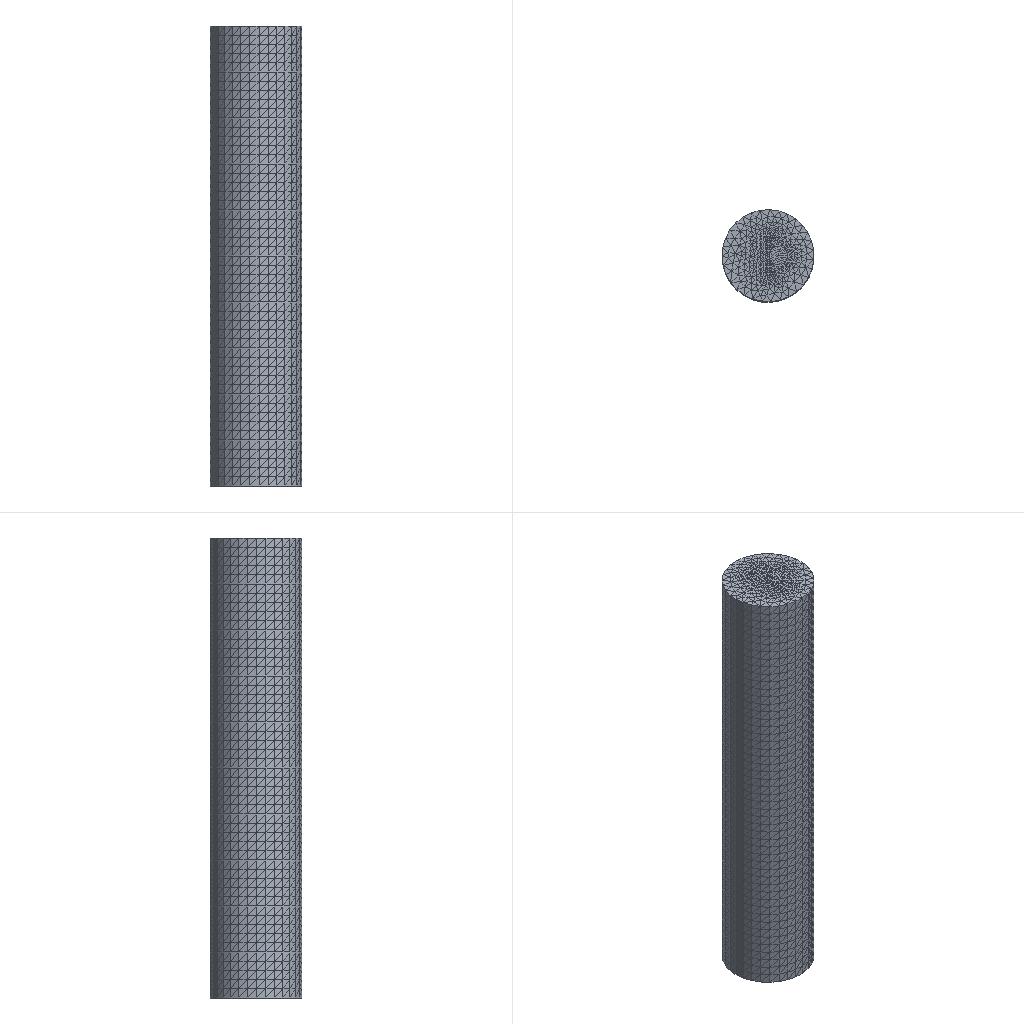Simulation study | abaqus
Set-up summary:
category,name,step,type,value,unit,region
solver,abaqus
solver,version,,,Abaqus/Explicit 2020
units,not stated in the deck,,not stated
analysis,deck,,transient,transient
load_step,Step-1,Step-1,transient,nlgeom=True
contact,interactions,,,general=0 pairs=0 ties=1
load_step,requested,,,1
mesh,nodes,,,13937
mesh,elements,,,62317
element_type,S3,,shell,32
element_type,S4R,,shell,2492
element_type,C3D4,,solid,59793
load,load commands in deck,,count,1
bc,support commands in deck,,count,4
material,BAN,,in results
material,MATERIAL-1,,in results
material,NANG,,in results
check,setup vs results,,match,"per instance, exact: element labels, types and connectivity; labels of the nodes the elements use; coordinates of those nodes at SINGLE_PRECISION in 1 of 5 instance(s)"
Abaqus input file, long lists of numbers shortened:
*Heading
** Job name: Job-2 Model name: Model-1-Copy
** Generated by: Abaqus/CAE 2020
*Preprint, echo=NO, model=NO, history=NO, contact=NO
**
** PARTS
**
*Part, name=qiao
*Node
      1, 0.02, -0.1,           0.
      2, 0.02,           0.,           0.
** (627 more lines like these left out)
*Element, type=S4R
  1,   1,  28,  78,  29
  2,  28,  27,  79,  78
** (621 more lines like these left out)
*Element, type=S3
501, 554,  66,  65
502, 578, 556, 567
** (6 more lines like these left out)
*Nset, nset=Set-1, generate
   1,  629,    1
*Elset, elset=Set-1, generate
   1,  631,    1
** Section: nang
*Shell Section, elset=Set-1, material=nang
0.001, 5
*End Part
**
*Part, name=tu-final
*Node
      1, 0.002, -0.05,           1.
      2, -0.002, -0.05,           1.
** (11419 more lines like these left out)
*Element, type=C3D4
   1, 948, 702, 956, 937
   2, 948, 912, 744, 897
** (59791 more lines like these left out)
*Nset, nset=Set-10
    1,    2,    3,    4,    5,    6,    7,    8,    9,   10,   11,   12,   13,   14,   15,   16
   20,   21,   22,   23,   25,   26,   27,   28,   29,   30,   31,   32,   33,   34,   35,   36
** (109 more lines like these left out)
*Elset, elset=Set-10
     1,     2,     3,     4,     5,     6,     7,     8,     9,    10,    11,    12,    13,    14,    15,    16
    17,    18,    19,    20,    21,    22,    23,    24,    25,    26,    27,    28,    29,    30,    31,    32
** (336 more lines like these left out)
*Nset, nset=Set-11
     1,     2,     3,     4,     5,     6,     7,     8,     9,    10,    11,    12,    13,    14,    15,    16
    17,    18,    19,    20,    21,    22,    23,    24,    25,    26,    27,    28,    29,    30,    31,    32
** (701 more lines like these left out)
*Elset, elset=Set-11
  1332,  1333,  1334,  1335,  1336,  1337,  1338,  1339,  1340,  1341,  1342,  1343,  1344,  1345,  1346,  1347
  1348,  1349,  1350,  1351,  1352,  1353,  1354,  1355,  1356,  1357,  1358,  1359,  1360,  1361,  1362,  1363
** (3398 more lines like these left out)
** Section: ban
*Solid Section, elset=Set-10, material=ban
,
** Section: tu
*Solid Section, elset=Set-11, material=Material-1
,
*End Part
**
**
** ASSEMBLY
**
*Assembly, name=Assembly
**
*Instance, name=tu-final-1, part=tu-final
*End Instance
**
*Instance, name=qiao-1, part=qiao
      -0.022,           0.,          0.6
      -0.022,           0.,          0.6, 0.978,           0.,          0.6, 90.
*End Instance
**
*Instance, name=qiao-2, part=qiao
       0.022,           0.,        0.735
       0.022,           0.,        0.735, 1.022,           0.,        0.735, 90.
*End Instance
**
*Instance, name=qiao-3, part=qiao
      -0.022,           0.,        0.865
      -0.022,           0.,        0.865, 0.978,           0.,        0.865, 90.
*End Instance
**
*Instance, name=qiao-4, part=qiao
       0.022,           0.,           1.
       0.022,           0.,           1., 1.022,           0.,           1., 90.
*End Instance
**
*Nset, nset=Set-1, instance=tu-final-1, generate
     1,  11421,      1
*Elset, elset=Set-1, instance=tu-final-1, generate
     1,  59793,      1
*Nset, nset=Set-2, instance=tu-final-1
    1,    2,    7,   14,   15,   19,   77,   78,   79,   80,   81,   82,   83,   84,   85,   86
   87,   88,   89,   90,   91,   92,   93,   94,   95,  165,  166,  167,  168,  169,  170,  171
** (22 more lines like these left out)
*Nset, nset=Set-2, instance=qiao-4
   2,   3,  48,  49,  50,  51,  52,  53,  54,  55,  56,  57,  58,  59,  60,  61
  62,  63,  64,  65,  66,  67,  68,  69,  70,  71,  72,  73,  74, 534, 535, 536
** (3 more lines like these left out)
*Elset, elset=Set-2, instance=tu-final-1
    82,   170,   172,   176,   178,   180,   186,   187,   190,   193,   199,   206,   215,   224,   225,   247
   480,   513,   518,   521,   522,   533,   540,   549,   943,   944,   945,   946,   948,   951,   955,  1162
** (43 more lines like these left out)
*Elset, elset=Set-2, instance=qiao-4, generate
 501,  566,    1
*Nset, nset=Set-3, instance=tu-final-1
   18,   19,   24,  380,  381,  382,  383,  384,  385,  386,  387,  388,  389,  390,  391,  392
  393,  394,  395,  396,  397,  398,  399,  400,  401,  402,  403,  404,  405,  406,  407,  408
** (97 more lines like these left out)
*Elset, elset=Set-3, instance=tu-final-1
  1501,  1518,  1522,  1611,  1732,  2047,  2048,  2127,  2307,  2332,  2374,  2402,  2519,  2636,  2656,  2775
  2805,  2883,  2936,  2943,  2954,  2999,  3025,  3061,  3154,  3214,  3347,  3639,  3763,  3981,  4015,  4021
** (192 more lines like these left out)
*Nset, nset=Set-4, instance=tu-final-1
    1,    2,    7,   14,   15,   19,   77,   78,   79,   80,   81,   82,   83,   84,   85,   86
   87,   88,   89,   90,   91,   92,   93,   94,   95,  165,  166,  167,  168,  169,  170,  171
** (22 more lines like these left out)
*Elset, elset=Set-4, instance=tu-final-1
    82,   170,   172,   176,   178,   180,   186,   187,   190,   193,   199,   206,   215,   224,   225,   247
   480,   513,   518,   521,   522,   533,   540,   549,   943,   944,   945,   946,   948,   951,   955,  1162
** (43 more lines like these left out)
*Nset, nset=Set-5, instance=qiao-4
   2,   3,  48,  49,  50,  51,  52,  53,  54,  55,  56,  57,  58,  59,  60,  61
  62,  63,  64,  65,  66,  67,  68,  69,  70,  71,  72,  73,  74, 534, 535, 536
** (3 more lines like these left out)
*Elset, elset=Set-5, instance=qiao-4, generate
 501,  566,    1
*Nset, nset=Set-6, instance=tu-final-1
   18,   19,   24,  380,  381,  382,  383,  384,  385,  386,  387,  388,  389,  390,  391,  392
  393,  394,  395,  396,  397,  398,  399,  400,  401,  402,  403,  404,  405,  406,  407,  408
** (97 more lines like these left out)
*Elset, elset=Set-6, instance=tu-final-1
  1501,  1518,  1522,  1611,  1732,  2047,  2048,  2127,  2307,  2332,  2374,  2402,  2519,  2636,  2656,  2775
  2805,  2883,  2936,  2943,  2954,  2999,  3025,  3061,  3154,  3214,  3347,  3639,  3763,  3981,  4015,  4021
** (192 more lines like these left out)
*Elset, elset=_Surf-3_SNEG, internal, instance=qiao-1, generate
   1,  500,    1
*Elset, elset=_Surf-3_SNEG, internal, instance=qiao-2, generate
   1,  500,    1
*Elset, elset=_Surf-3_SNEG, internal, instance=qiao-4, generate
   1,  500,    1
*Elset, elset=_Surf-3_SNEG, internal, instance=qiao-3, generate
   1,  500,    1
*Surface, type=ELEMENT, name=Surf-3
_Surf-3_SNEG, SNEG
*Elset, elset=_m_Surf-1_S4, internal, instance=tu-final-1
  1660,  1956,  1968,  1981,  2150,  2284,  2349,  2375,  2422,  3932,  5160,  5327,  5356,  5400,  5516,  5620
  5644,  5672,  5699,  5713,  5720,  5730,  5848,  5918,  5922,  5957,  6049,  6102,  6250,  6274,  6315,  6433
** (15 more lines like these left out)
*Elset, elset=_m_Surf-1_S3, internal, instance=tu-final-1
  1441,  1751,  1760,  2099,  2493,  2703,  2704,  2827,  2941,  3142,  3221,  3312,  3332,  3392,  3429,  3644
  3780,  3855,  3967,  4007,  4252,  5074,  5075,  5084,  5117,  5140,  5168,  5172,  5182,  5186,  5190,  5212
** (81 more lines like these left out)
*Elset, elset=_m_Surf-1_S2, internal, instance=tu-final-1
  1384,  4371,  5082,  5107,  5131,  5197,  5381,  5518,  5561,  5586,  5628,  5632,  5710,  5798,  5808,  5978
  5999,  6064,  6206,  6212,  6236,  6282,  6334,  6340,  6367,  6409,  6683,  6746,  6770,  6852,  6916,  7000
** (8 more lines like these left out)
*Elset, elset=_m_Surf-1_S1, internal, instance=tu-final-1
  1772,  1958,  2088,  2128,  2226,  3905,  4678,  4763,  5694,  5890,  5990,  5996,  6038,  6495,  6610,  6718
  6872,  7364,  7367,  7573,  7883,  7980,  8002,  8164,  8171,  8352,  9342,  9366,  9845, 10036, 10052, 10100
** (5 more lines like these left out)
*Surface, type=ELEMENT, name=m_Surf-1
_m_Surf-1_S4, S4
_m_Surf-1_S3, S3
_m_Surf-1_S2, S2
_m_Surf-1_S1, S1
*Elset, elset=_s_Surf-1_SPOS, internal, instance=qiao-1, generate
   1,  631,    1
*Elset, elset=_s_Surf-1_SPOS, internal, instance=qiao-2, generate
   1,  631,    1
*Elset, elset=_s_Surf-1_SPOS, internal, instance=qiao-4, generate
   1,  631,    1
*Elset, elset=_s_Surf-1_SPOS, internal, instance=qiao-3, generate
   1,  631,    1
*Surface, type=ELEMENT, name=s_Surf-1
_s_Surf-1_SPOS, SPOS
** Constraint: Constraint-1
*Tie, name=Constraint-1, adjust=yes
s_Surf-1, m_Surf-1
*End Assembly
*Amplitude, name=Amp-1
             0.,              0.,             0.5,              1.,              1.,              0.
**
** MATERIALS
**
*Material, name=Material-1
*Density
2200.,
*Elastic
 5e+08, 0.35
*Mohr Coulomb
22., 0.1
*Mohr Coulomb Hardening
150000.,0.
*Material, name=ban
*Density
1200.,
*Elastic
 1.3e+10, 0.35
*Material, name=nang
*Density
1100.,
*Hyperelastic, mooney-rivlin
 0.805, 0.194,    0.
**
** INTERACTION PROPERTIES
**
*Surface Interaction, name=IntProp-1
*Friction
 0.1,
*Surface Behavior, pressure-overclosure=HARD
**
** PREDEFINED FIELDS
**
** Name: Predefined Field-2   Type: Stress
*Initial Conditions, type=STRESS
tu-final-1.Set-11, -100000., -100000., -100000., -100000., -100000., -100000.
** ----------------------------------------------------------------
**
** STEP: Step-1
**
*Step, name=Step-1, nlgeom=YES
*Dynamic, Explicit
, 1.
*Bulk Viscosity
0.06, 1.2
** Mass Scaling: Semi-Automatic
**               Whole Model
*Fixed Mass Scaling, factor=5000.
**
** BOUNDARY CONDITIONS
**
** Name: BC-1 Type: 对称/反对称/完全固定
*Boundary
Set-4, ENCASTRE
** Name: BC-3 Type: 位移/转角
*Boundary
Set-5, 3, 3
** Name: [REDACTED] : Displacement/rotation angle
*Boundary
Set-3, 1, 1
Set-3, 2, 2
**
** LOADS
**
** Name: Load-1   Type: Pressure
*Dsload
Surf-3, P, 1e+07
**
** OUTPUT REQUESTS
**
*Restart, write, number interval=1, time marks=NO
**
** FIELD OUTPUT: F-Output-1
**
*Output, field, number interval=50
*Node Output
CF, POR, RF, RM, RT, U, UR, UT
V, VR, VT
*Element Output, directions=YES
E, LE, MISES, MISESMAX, PE, PEEQ, PEEQT, PEMAG, S, SEQUT, SF, YIELDPOT
*Contact Output
CDISP, CSTRESS
**
** HISTORY OUTPUT: H-Output-1
**
*Output, history, variable=PRESELECT, frequency=1
*End Step
Results summary:
result,step,Step-1,completed,increments=55603 time=1.0/1.0
result,analysis,,,transient
result,last_loadstep,,,1
result,analysis steps,,count,1
result,primary field,,,"U, UR"
result,reaction total,,FX,5564.607,model units
result,reaction total,,FY,-41.542,model units
result,reaction total,,FZ,14360.341,model units